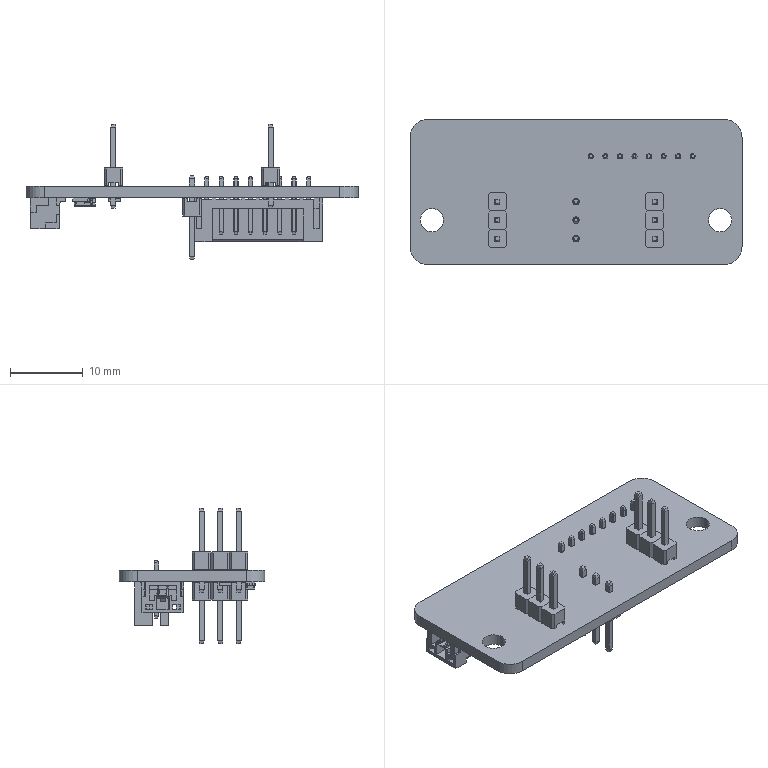Part | NX | features BREP 177 | 177 solids | 2193 faces | box 45.595 x 20 x 18.599 mm | volume 1843 mm3 | plane 1417 | spline 448 | cylinder 324 | sphere 4 | commonest cylinder face diameters 0.1 x102 0.06 x54 0.011 x18 0.39 x18 0.45 x18 0.9 x18